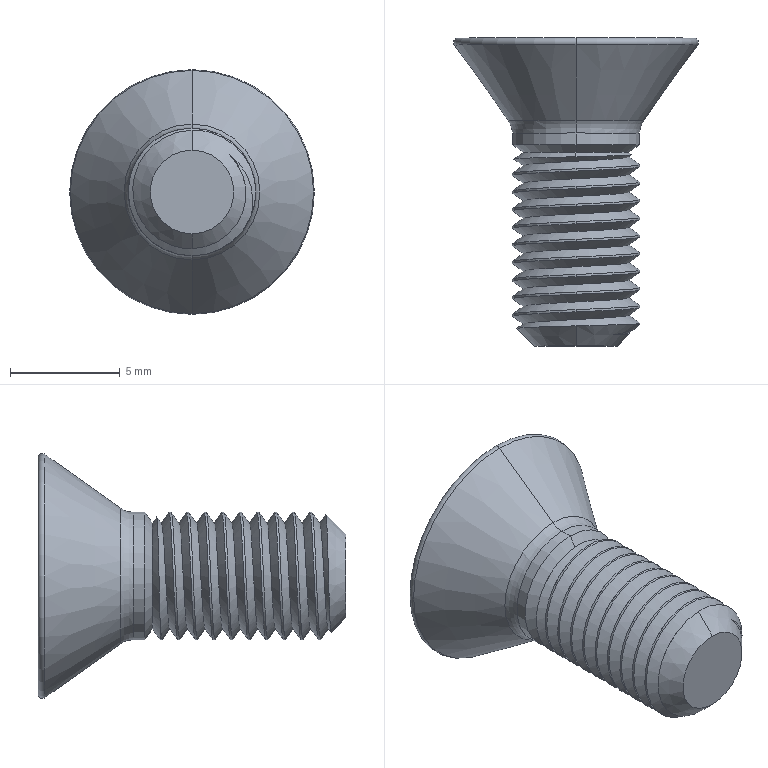Part | STEP file | Screw M6 - 10mm flat head | 1 solid | 45 faces | box 11.124 x 14 x 11.124 mm | volume 424.589 mm3 | cylinder 22 | plane 9 | cone 8 | torus 4 | spline 2 | commonest cylinder face diameters 5.8 x22